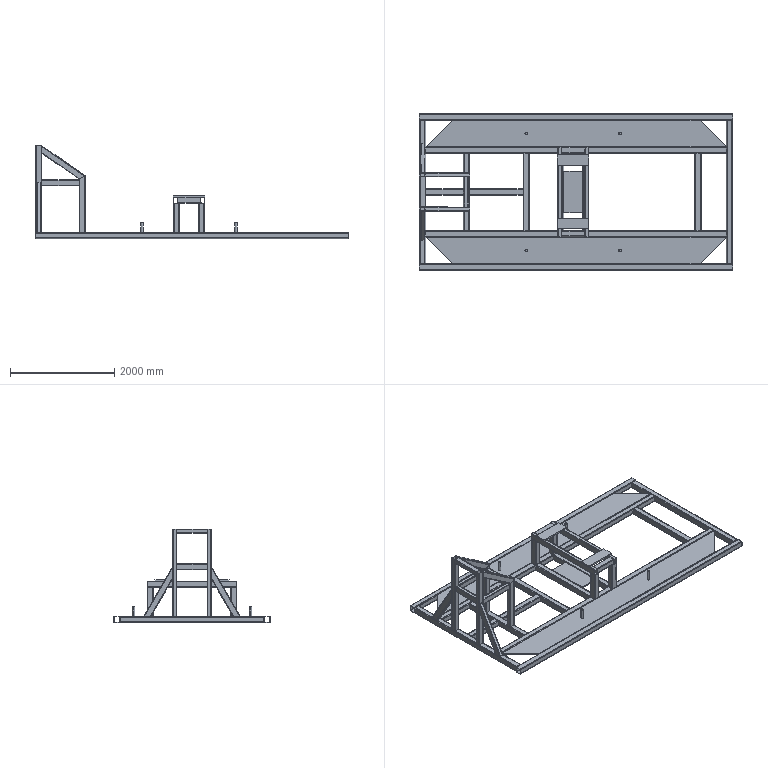Part | SolidWorks | features WeldCornerFeat 9, ICE 4, MoveCopyBody 4, WeldMemberFeat 3, MirrorSolid 2, 3DProfileFeature 1, LPattern 1, WeldmentFeature 1 | 43 solids | 666 faces | box 6000 x 3000 x 1795 mm | volume 349583429 mm3 | plane 378 | cylinder 288 | commonest cylinder face diameters 16 x76 32 x76 12 x60 24 x60 40 x8 48 x8